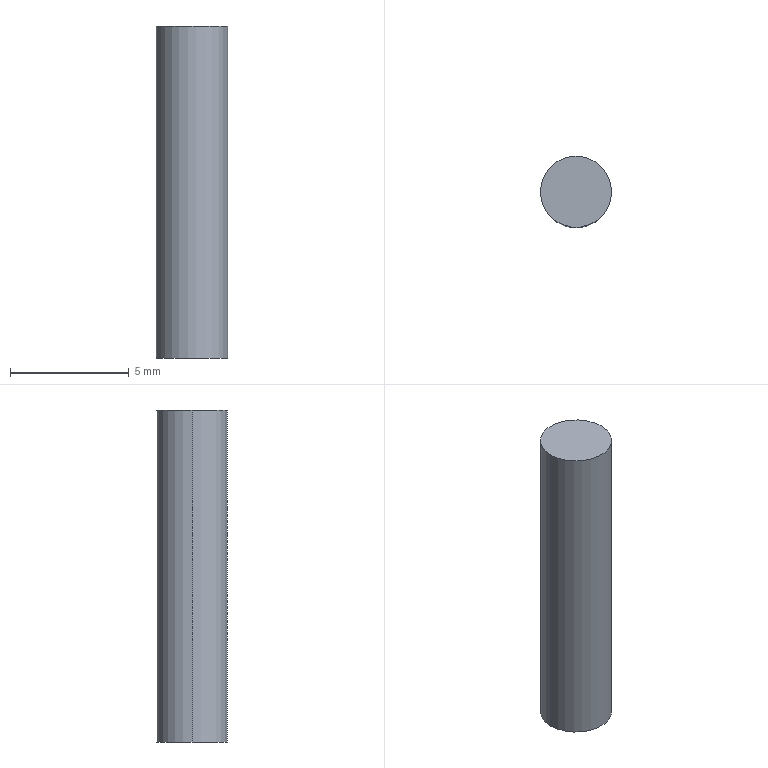Part | STEP file | push magnet block pin | 1 solid | 4 faces | box 3 x 3 x 14 mm | volume 98.96 mm3 | cylinder 2 | plane 2 | commonest cylinder face diameters 3 x2
STEP:
#1=CARTESIAN_POINT('',(0.,0.,0.));
#2=DIRECTION('',(0.,0.,1.));
#3=DIRECTION('',(1.,0.,0.));
#4=AXIS2_PLACEMENT_3D('',#1,#2,#3);
#5=CARTESIAN_POINT('',(1.5,0.,14.));
#6=VERTEX_POINT('',#5);
#7=CARTESIAN_POINT('',(-1.5,0.,14.));
#8=VERTEX_POINT('',#7);
#9=CARTESIAN_POINT('',(0.,0.,14.));
#10=DIRECTION('',(0.,0.,1.));
#11=DIRECTION('',(1.,0.,0.));
#12=AXIS2_PLACEMENT_3D('',#9,#10,#11);
#13=CIRCLE('',#12,1.5);
#14=CARTESIAN_POINT('',(0.,0.,14.));
#15=DIRECTION('',(0.,0.,-1.));
#16=DIRECTION('',(-1.,0.,0.));
#17=AXIS2_PLACEMENT_3D('',#14,#15,#16);
#18=CYLINDRICAL_SURFACE('',#17,1.5);
#19=CARTESIAN_POINT('',(3.142,0.));
#20=DIRECTION('',(-1.,0.));
#21=VECTOR('',#20,1.);
#22=LINE('',#19,#21);
#23=(GEOMETRIC_REPRESENTATION_CONTEXT(2)PARAMETRIC_REPRESENTATION_CONTEXT()REPRESENTATION_CONTEXT('',''));
#24=DEFINITIONAL_REPRESENTATION('',(#22),#23);
#25=PCURVE('',#18,#24);
#26=CARTESIAN_POINT('',(0.,0.,14.));
#27=DIRECTION('',(0.,0.,1.));
#28=DIRECTION('',(1.,0.,0.));
#29=AXIS2_PLACEMENT_3D('',#26,#27,#28);
#30=PLANE('',#29);
#31=CARTESIAN_POINT('',(0.,0.));
#32=DIRECTION('',(1.,0.));
#33=AXIS2_PLACEMENT_2D('',#31,#32);
#34=CIRCLE('',#33,1.5);
#35=(GEOMETRIC_REPRESENTATION_CONTEXT(2)PARAMETRIC_REPRESENTATION_CONTEXT()REPRESENTATION_CONTEXT('',''));
#36=DEFINITIONAL_REPRESENTATION('',(#34),#35);
#37=PCURVE('',#30,#36);
#38=SURFACE_CURVE('',#13,(#25,#37),.PCURVE_S1.);
#39=EDGE_CURVE('',#6,#8,#38,.T.);
#40=ORIENTED_EDGE('',*,*,#39,.F.);
#41=CARTESIAN_POINT('',(1.5,0.,0.));
#42=VERTEX_POINT('',#41);
#43=CARTESIAN_POINT('',(1.5,0.,14.));
#44=DIRECTION('',(0.,0.,-1.));
#45=VECTOR('',#44,1.);
#46=LINE('',#43,#45);
#47=CARTESIAN_POINT('',(3.142,0.));
#48=DIRECTION('',(0.,1.));
#49=VECTOR('',#48,1.);
#50=LINE('',#47,#49);
#51=(GEOMETRIC_REPRESENTATION_CONTEXT(2)PARAMETRIC_REPRESENTATION_CONTEXT()REPRESENTATION_CONTEXT('',''));
#52=DEFINITIONAL_REPRESENTATION('',(#50),#51);
#53=PCURVE('',#18,#52);
#54=CARTESIAN_POINT('',(0.,0.,14.));
#55=DIRECTION('',(0.,0.,-1.));
#56=DIRECTION('',(-1.,0.,0.));
#57=AXIS2_PLACEMENT_3D('',#54,#55,#56);
#58=CYLINDRICAL_SURFACE('',#57,1.5);
#59=CARTESIAN_POINT('',(3.142,0.));
#60=DIRECTION('',(0.,1.));
#61=VECTOR('',#60,1.);
#62=LINE('',#59,#61);
#63=(GEOMETRIC_REPRESENTATION_CONTEXT(2)PARAMETRIC_REPRESENTATION_CONTEXT()REPRESENTATION_CONTEXT('',''));
#64=DEFINITIONAL_REPRESENTATION('',(#62),#63);
#65=PCURVE('',#58,#64);
#66=SURFACE_CURVE('',#46,(#53,#65),.PCURVE_S1.);
#67=EDGE_CURVE('',#6,#42,#66,.T.);
#68=ORIENTED_EDGE('',*,*,#67,.T.);
#69=CARTESIAN_POINT('',(-1.5,0.,0.));
#70=VERTEX_POINT('',#69);
#71=CARTESIAN_POINT('',(0.,0.,0.));
#72=DIRECTION('',(0.,0.,1.));
#73=DIRECTION('',(1.,0.,0.));
#74=AXIS2_PLACEMENT_3D('',#71,#72,#73);
#75=CIRCLE('',#74,1.5);
#76=CARTESIAN_POINT('',(3.142,14.));
#77=DIRECTION('',(-1.,0.));
#78=VECTOR('',#77,1.);
#79=LINE('',#76,#78);
#80=(GEOMETRIC_REPRESENTATION_CONTEXT(2)PARAMETRIC_REPRESENTATION_CONTEXT()REPRESENTATION_CONTEXT('',''));
#81=DEFINITIONAL_REPRESENTATION('',(#79),#80);
#82=PCURVE('',#18,#81);
#83=CARTESIAN_POINT('',(0.,0.,0.));
#84=DIRECTION('',(0.,0.,1.));
#85=DIRECTION('',(1.,0.,0.));
#86=AXIS2_PLACEMENT_3D('',#83,#84,#85);
#87=PLANE('',#86);
#88=CARTESIAN_POINT('',(0.,0.));
#89=DIRECTION('',(1.,0.));
#90=AXIS2_PLACEMENT_2D('',#88,#89);
#91=CIRCLE('',#90,1.5);
#92=(GEOMETRIC_REPRESENTATION_CONTEXT(2)PARAMETRIC_REPRESENTATION_CONTEXT()REPRESENTATION_CONTEXT('',''));
#93=DEFINITIONAL_REPRESENTATION('',(#91),#92);
#94=PCURVE('',#87,#93);
#95=SURFACE_CURVE('',#75,(#82,#94),.PCURVE_S1.);
#96=EDGE_CURVE('',#42,#70,#95,.T.);
#97=ORIENTED_EDGE('',*,*,#96,.T.);
#98=CARTESIAN_POINT('',(-1.5,0.,14.));
#99=DIRECTION('',(0.,0.,-1.));
#100=VECTOR('',#99,1.);
#101=LINE('',#98,#100);
#102=CARTESIAN_POINT('',(0.,0.));
#103=DIRECTION('',(0.,1.));
#104=VECTOR('',#103,1.);
#105=LINE('',#102,#104);
#106=(GEOMETRIC_REPRESENTATION_CONTEXT(2)PARAMETRIC_REPRESENTATION_CONTEXT()REPRESENTATION_CONTEXT('',''));
#107=DEFINITIONAL_REPRESENTATION('',(#105),#106);
#108=PCURVE('',#18,#107);
#109=CARTESIAN_POINT('',(6.283,0.));
#110=DIRECTION('',(0.,1.));
#111=VECTOR('',#110,1.);
#112=LINE('',#109,#111);
#113=(GEOMETRIC_REPRESENTATION_CONTEXT(2)PARAMETRIC_REPRESENTATION_CONTEXT()REPRESENTATION_CONTEXT('',''));
#114=DEFINITIONAL_REPRESENTATION('',(#112),#113);
#115=PCURVE('',#58,#114);
#116=SURFACE_CURVE('',#101,(#108,#115),.PCURVE_S1.);
#117=EDGE_CURVE('',#8,#70,#116,.T.);
#118=ORIENTED_EDGE('',*,*,#117,.F.);
#119=EDGE_LOOP('',(#40,#68,#97,#118));
#120=FACE_BOUND('',#119,.T.);
#121=ADVANCED_FACE('',(#120),#18,.T.);
#122=ORIENTED_EDGE('',*,*,#67,.F.);
#123=CARTESIAN_POINT('',(0.,0.,14.));
#124=DIRECTION('',(0.,0.,1.));
#125=DIRECTION('',(1.,0.,0.));
#126=AXIS2_PLACEMENT_3D('',#123,#124,#125);
#127=CIRCLE('',#126,1.5);
#128=CARTESIAN_POINT('',(9.425,0.));
#129=DIRECTION('',(-1.,0.));
#130=VECTOR('',#129,1.);
#131=LINE('',#128,#130);
#132=(GEOMETRIC_REPRESENTATION_CONTEXT(2)PARAMETRIC_REPRESENTATION_CONTEXT()REPRESENTATION_CONTEXT('',''));
#133=DEFINITIONAL_REPRESENTATION('',(#131),#132);
#134=PCURVE('',#58,#133);
#135=CARTESIAN_POINT('',(0.,0.));
#136=DIRECTION('',(1.,0.));
#137=AXIS2_PLACEMENT_2D('',#135,#136);
#138=CIRCLE('',#137,1.5);
#139=(GEOMETRIC_REPRESENTATION_CONTEXT(2)PARAMETRIC_REPRESENTATION_CONTEXT()REPRESENTATION_CONTEXT('',''));
#140=DEFINITIONAL_REPRESENTATION('',(#138),#139);
#141=PCURVE('',#30,#140);
#142=SURFACE_CURVE('',#127,(#134,#141),.PCURVE_S1.);
#143=EDGE_CURVE('',#8,#6,#142,.T.);
#144=ORIENTED_EDGE('',*,*,#143,.F.);
#145=ORIENTED_EDGE('',*,*,#117,.T.);
#146=CARTESIAN_POINT('',(0.,0.,0.));
#147=DIRECTION('',(0.,0.,1.));
#148=DIRECTION('',(1.,0.,0.));
#149=AXIS2_PLACEMENT_3D('',#146,#147,#148);
#150=CIRCLE('',#149,1.5);
#151=CARTESIAN_POINT('',(9.425,14.));
#152=DIRECTION('',(-1.,0.));
#153=VECTOR('',#152,1.);
#154=LINE('',#151,#153);
#155=(GEOMETRIC_REPRESENTATION_CONTEXT(2)PARAMETRIC_REPRESENTATION_CONTEXT()REPRESENTATION_CONTEXT('',''));
#156=DEFINITIONAL_REPRESENTATION('',(#154),#155);
#157=PCURVE('',#58,#156);
#158=CARTESIAN_POINT('',(0.,0.));
#159=DIRECTION('',(1.,0.));
#160=AXIS2_PLACEMENT_2D('',#158,#159);
#161=CIRCLE('',#160,1.5);
#162=(GEOMETRIC_REPRESENTATION_CONTEXT(2)PARAMETRIC_REPRESENTATION_CONTEXT()REPRESENTATION_CONTEXT('',''));
#163=DEFINITIONAL_REPRESENTATION('',(#161),#162);
#164=PCURVE('',#87,#163);
#165=SURFACE_CURVE('',#150,(#157,#164),.PCURVE_S1.);
#166=EDGE_CURVE('',#70,#42,#165,.T.);
#167=ORIENTED_EDGE('',*,*,#166,.T.);
#168=EDGE_LOOP('',(#122,#144,#145,#167));
#169=FACE_BOUND('',#168,.T.);
#170=ADVANCED_FACE('',(#169),#58,.T.);
#171=ORIENTED_EDGE('',*,*,#143,.T.);
#172=ORIENTED_EDGE('',*,*,#39,.T.);
#173=EDGE_LOOP('',(#171,#172));
#174=FACE_BOUND('',#173,.T.);
#175=ADVANCED_FACE('',(#174),#30,.T.);
#176=ORIENTED_EDGE('',*,*,#166,.F.);
#177=ORIENTED_EDGE('',*,*,#96,.F.);
#178=EDGE_LOOP('',(#176,#177));
#179=FACE_BOUND('',#178,.T.);
#180=ADVANCED_FACE('',(#179),#87,.F.);
#181=CLOSED_SHELL('',(#121,#170,#175,#180));
#182=MANIFOLD_SOLID_BREP('',#181);
#183=(LENGTH_UNIT()NAMED_UNIT(*)SI_UNIT(.MILLI.,.METRE.));
#184=UNCERTAINTY_MEASURE_WITH_UNIT(LENGTH_MEASURE(0.0000001),#183,'','');
#185=(NAMED_UNIT(*)PLANE_ANGLE_UNIT()SI_UNIT($,.RADIAN.));
#186=(NAMED_UNIT(*)SI_UNIT($,.STERADIAN.)SOLID_ANGLE_UNIT());
#187=(GEOMETRIC_REPRESENTATION_CONTEXT(3)GLOBAL_UNCERTAINTY_ASSIGNED_CONTEXT((#184))GLOBAL_UNIT_ASSIGNED_CONTEXT((#183,#185,#186))REPRESENTATION_CONTEXT('',''));
#188=ADVANCED_BREP_SHAPE_REPRESENTATION('',(#4,#182),#187);